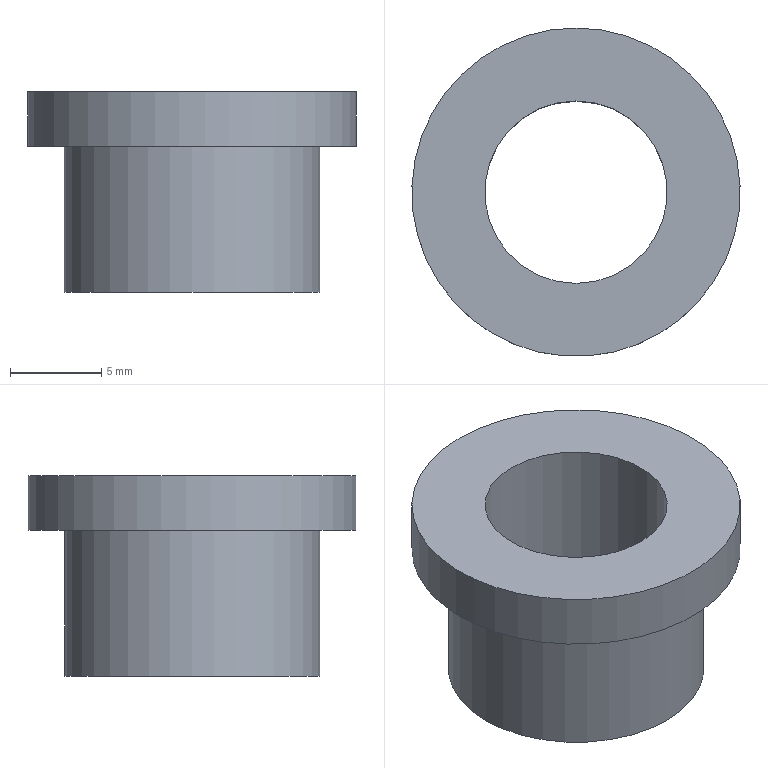Part | STEP file | 1-58A | 1 solid | 6 faces | box 18 x 18 x 11 mm | volume 1131 mm3 | plane 3 | cylinder 3 | commonest cylinder face diameters 10 x1 14 x1 18 x1
STEP:
#1=CARTESIAN_POINT('',(0.,0.,0.));
#2=DIRECTION('',(0.,0.,1.));
#3=DIRECTION('',(1.,0.,0.));
#4=AXIS2_PLACEMENT_3D('',#1,#2,#3);
#5=CARTESIAN_POINT('',(0.,7.,-8.));
#6=VERTEX_POINT('',#5);
#7=CARTESIAN_POINT('',(0.,0.,-8.));
#8=DIRECTION('',(0.,0.,1.));
#9=DIRECTION('',(0.,1.,0.));
#10=AXIS2_PLACEMENT_3D('',#7,#8,#9);
#11=CIRCLE('',#10,7.);
#12=CARTESIAN_POINT('',(0.,-1.876,-8.));
#13=DIRECTION('',(0.,0.,1.));
#14=DIRECTION('',(1.,0.,0.));
#15=AXIS2_PLACEMENT_3D('',#12,#13,#14);
#16=PLANE('',#15);
#17=CARTESIAN_POINT('',(0.,1.876));
#18=DIRECTION('',(0.,1.));
#19=AXIS2_PLACEMENT_2D('',#17,#18);
#20=CIRCLE('',#19,7.);
#21=(GEOMETRIC_REPRESENTATION_CONTEXT(2)PARAMETRIC_REPRESENTATION_CONTEXT()REPRESENTATION_CONTEXT('',''));
#22=DEFINITIONAL_REPRESENTATION('',(#20),#21);
#23=PCURVE('',#16,#22);
#24=CARTESIAN_POINT('',(0.,0.,0.));
#25=DIRECTION('',(0.,0.,-1.));
#26=DIRECTION('',(0.,1.,0.));
#27=AXIS2_PLACEMENT_3D('',#24,#25,#26);
#28=CYLINDRICAL_SURFACE('',#27,7.);
#29=CARTESIAN_POINT('',(6.283,8.));
#30=DIRECTION('',(-1.,0.));
#31=VECTOR('',#30,1.);
#32=LINE('',#29,#31);
#33=(GEOMETRIC_REPRESENTATION_CONTEXT(2)PARAMETRIC_REPRESENTATION_CONTEXT()REPRESENTATION_CONTEXT('',''));
#34=DEFINITIONAL_REPRESENTATION('',(#32),#33);
#35=PCURVE('',#28,#34);
#36=SURFACE_CURVE('',#11,(#23,#35),.PCURVE_S1.);
#37=EDGE_CURVE('',#6,#6,#36,.T.);
#38=ORIENTED_EDGE('',*,*,#37,.T.);
#39=EDGE_LOOP('',(#38));
#40=FACE_BOUND('',#39,.F.);
#41=CARTESIAN_POINT('',(0.,5.,-8.));
#42=VERTEX_POINT('',#41);
#43=CARTESIAN_POINT('',(0.,0.,-8.));
#44=DIRECTION('',(0.,0.,-1.));
#45=DIRECTION('',(0.,1.,0.));
#46=AXIS2_PLACEMENT_3D('',#43,#44,#45);
#47=CIRCLE('',#46,5.);
#48=CARTESIAN_POINT('',(0.,6.876));
#49=CARTESIAN_POINT('',(8.66,6.876));
#50=CARTESIAN_POINT('',(4.33,-0.6244));
#51=CARTESIAN_POINT('',(0.,-8.124));
#52=CARTESIAN_POINT('',(-4.33,-0.6244));
#53=CARTESIAN_POINT('',(-8.66,6.876));
#54=CARTESIAN_POINT('',(0.,6.876));
#55=(BOUNDED_CURVE()B_SPLINE_CURVE(2,(#48,#49,#50,#51,#52,#53,#54),.UNSPECIFIED.,.T.,.F.)B_SPLINE_CURVE_WITH_KNOTS((1,2,2,2,2,1),(-2.094,0.,2.094,4.189,6.283,8.378),.UNSPECIFIED.)CURVE()GEOMETRIC_REPRESENTATION_ITEM()RATIONAL_B_SPLINE_CURVE((1.,0.5,1.,0.5,1.,0.5,1.))REPRESENTATION_ITEM(''));
#56=(GEOMETRIC_REPRESENTATION_CONTEXT(2)PARAMETRIC_REPRESENTATION_CONTEXT()REPRESENTATION_CONTEXT('',''));
#57=DEFINITIONAL_REPRESENTATION('',(#55),#56);
#58=PCURVE('',#16,#57);
#59=CARTESIAN_POINT('',(0.,0.,3.));
#60=DIRECTION('',(0.,0.,-1.));
#61=DIRECTION('',(0.,1.,0.));
#62=AXIS2_PLACEMENT_3D('',#59,#60,#61);
#63=CYLINDRICAL_SURFACE('',#62,5.);
#64=CARTESIAN_POINT('',(0.,11.));
#65=DIRECTION('',(1.,0.));
#66=VECTOR('',#65,1.);
#67=LINE('',#64,#66);
#68=(GEOMETRIC_REPRESENTATION_CONTEXT(2)PARAMETRIC_REPRESENTATION_CONTEXT()REPRESENTATION_CONTEXT('',''));
#69=DEFINITIONAL_REPRESENTATION('',(#67),#68);
#70=PCURVE('',#63,#69);
#71=SURFACE_CURVE('',#47,(#58,#70),.PCURVE_S1.);
#72=EDGE_CURVE('',#42,#42,#71,.T.);
#73=ORIENTED_EDGE('',*,*,#72,.T.);
#74=EDGE_LOOP('',(#73));
#75=FACE_BOUND('',#74,.F.);
#76=ADVANCED_FACE('',(#40,#75),#16,.F.);
#77=CARTESIAN_POINT('',(0.,7.,0.));
#78=VERTEX_POINT('',#77);
#79=CARTESIAN_POINT('',(0.,7.,0.));
#80=DIRECTION('',(0.,0.,-1.));
#81=VECTOR('',#80,1.);
#82=LINE('',#79,#81);
#83=CARTESIAN_POINT('',(6.283,0.));
#84=DIRECTION('',(0.,1.));
#85=VECTOR('',#84,1.);
#86=LINE('',#83,#85);
#87=(GEOMETRIC_REPRESENTATION_CONTEXT(2)PARAMETRIC_REPRESENTATION_CONTEXT()REPRESENTATION_CONTEXT('',''));
#88=DEFINITIONAL_REPRESENTATION('',(#86),#87);
#89=PCURVE('',#28,#88);
#90=CARTESIAN_POINT('',(0.,0.));
#91=DIRECTION('',(0.,1.));
#92=VECTOR('',#91,1.);
#93=LINE('',#90,#92);
#94=(GEOMETRIC_REPRESENTATION_CONTEXT(2)PARAMETRIC_REPRESENTATION_CONTEXT()REPRESENTATION_CONTEXT('',''));
#95=DEFINITIONAL_REPRESENTATION('',(#93),#94);
#96=PCURVE('',#28,#95);
#97=SEAM_CURVE('',#82,(#89,#96),.PCURVE_S1.);
#98=EDGE_CURVE('',#78,#6,#97,.T.);
#99=ORIENTED_EDGE('',*,*,#98,.T.);
#100=ORIENTED_EDGE('',*,*,#37,.T.);
#101=ORIENTED_EDGE('',*,*,#98,.F.);
#102=CARTESIAN_POINT('',(0.,0.,0.));
#103=DIRECTION('',(0.,0.,1.));
#104=DIRECTION('',(0.,1.,0.));
#105=AXIS2_PLACEMENT_3D('',#102,#103,#104);
#106=CIRCLE('',#105,7.);
#107=CARTESIAN_POINT('',(6.283,0.));
#108=DIRECTION('',(-1.,0.));
#109=VECTOR('',#108,1.);
#110=LINE('',#107,#109);
#111=(GEOMETRIC_REPRESENTATION_CONTEXT(2)PARAMETRIC_REPRESENTATION_CONTEXT()REPRESENTATION_CONTEXT('',''));
#112=DEFINITIONAL_REPRESENTATION('',(#110),#111);
#113=PCURVE('',#28,#112);
#114=CARTESIAN_POINT('',(0.,-2.412,0.));
#115=DIRECTION('',(0.,0.,1.));
#116=DIRECTION('',(1.,0.,0.));
#117=AXIS2_PLACEMENT_3D('',#114,#115,#116);
#118=PLANE('',#117);
#119=CARTESIAN_POINT('',(0.,2.412));
#120=DIRECTION('',(0.,1.));
#121=AXIS2_PLACEMENT_2D('',#119,#120);
#122=CIRCLE('',#121,7.);
#123=(GEOMETRIC_REPRESENTATION_CONTEXT(2)PARAMETRIC_REPRESENTATION_CONTEXT()REPRESENTATION_CONTEXT('',''));
#124=DEFINITIONAL_REPRESENTATION('',(#122),#123);
#125=PCURVE('',#118,#124);
#126=SURFACE_CURVE('',#106,(#113,#125),.PCURVE_S1.);
#127=EDGE_CURVE('',#78,#78,#126,.T.);
#128=ORIENTED_EDGE('',*,*,#127,.F.);
#129=EDGE_LOOP('',(#99,#100,#101,#128));
#130=FACE_BOUND('',#129,.T.);
#131=ADVANCED_FACE('',(#130),#28,.T.);
#132=ORIENTED_EDGE('',*,*,#72,.F.);
#133=CARTESIAN_POINT('',(0.,5.,3.));
#134=VERTEX_POINT('',#133);
#135=CARTESIAN_POINT('',(0.,5.,-8.));
#136=DIRECTION('',(0.,0.,1.));
#137=VECTOR('',#136,1.);
#138=LINE('',#135,#137);
#139=CARTESIAN_POINT('',(0.,11.));
#140=DIRECTION('',(0.,-1.));
#141=VECTOR('',#140,1.);
#142=LINE('',#139,#141);
#143=(GEOMETRIC_REPRESENTATION_CONTEXT(2)PARAMETRIC_REPRESENTATION_CONTEXT()REPRESENTATION_CONTEXT('',''));
#144=DEFINITIONAL_REPRESENTATION('',(#142),#143);
#145=PCURVE('',#63,#144);
#146=CARTESIAN_POINT('',(6.283,11.));
#147=DIRECTION('',(0.,-1.));
#148=VECTOR('',#147,1.);
#149=LINE('',#146,#148);
#150=(GEOMETRIC_REPRESENTATION_CONTEXT(2)PARAMETRIC_REPRESENTATION_CONTEXT()REPRESENTATION_CONTEXT('',''));
#151=DEFINITIONAL_REPRESENTATION('',(#149),#150);
#152=PCURVE('',#63,#151);
#153=SEAM_CURVE('',#138,(#145,#152),.PCURVE_S1.);
#154=EDGE_CURVE('',#42,#134,#153,.T.);
#155=ORIENTED_EDGE('',*,*,#154,.T.);
#156=CARTESIAN_POINT('',(0.,0.,3.));
#157=DIRECTION('',(0.,0.,-1.));
#158=DIRECTION('',(0.,1.,0.));
#159=AXIS2_PLACEMENT_3D('',#156,#157,#158);
#160=CIRCLE('',#159,5.);
#161=CARTESIAN_POINT('',(0.,0.));
#162=DIRECTION('',(1.,0.));
#163=VECTOR('',#162,1.);
#164=LINE('',#161,#163);
#165=(GEOMETRIC_REPRESENTATION_CONTEXT(2)PARAMETRIC_REPRESENTATION_CONTEXT()REPRESENTATION_CONTEXT('',''));
#166=DEFINITIONAL_REPRESENTATION('',(#164),#165);
#167=PCURVE('',#63,#166);
#168=CARTESIAN_POINT('',(0.,-2.412,3.));
#169=DIRECTION('',(0.,0.,1.));
#170=DIRECTION('',(1.,0.,0.));
#171=AXIS2_PLACEMENT_3D('',#168,#169,#170);
#172=PLANE('',#171);
#173=CARTESIAN_POINT('',(0.,7.412));
#174=CARTESIAN_POINT('',(8.66,7.412));
#175=CARTESIAN_POINT('',(4.33,-0.08846));
#176=CARTESIAN_POINT('',(0.,-7.588));
#177=CARTESIAN_POINT('',(-4.33,-0.08846));
#178=CARTESIAN_POINT('',(-8.66,7.412));
#179=CARTESIAN_POINT('',(0.,7.412));
#180=(BOUNDED_CURVE()B_SPLINE_CURVE(2,(#173,#174,#175,#176,#177,#178,#179),.UNSPECIFIED.,.T.,.F.)B_SPLINE_CURVE_WITH_KNOTS((1,2,2,2,2,1),(-2.094,0.,2.094,4.189,6.283,8.378),.UNSPECIFIED.)CURVE()GEOMETRIC_REPRESENTATION_ITEM()RATIONAL_B_SPLINE_CURVE((1.,0.5,1.,0.5,1.,0.5,1.))REPRESENTATION_ITEM(''));
#181=(GEOMETRIC_REPRESENTATION_CONTEXT(2)PARAMETRIC_REPRESENTATION_CONTEXT()REPRESENTATION_CONTEXT('',''));
#182=DEFINITIONAL_REPRESENTATION('',(#180),#181);
#183=PCURVE('',#172,#182);
#184=SURFACE_CURVE('',#160,(#167,#183),.PCURVE_S1.);
#185=EDGE_CURVE('',#134,#134,#184,.T.);
#186=ORIENTED_EDGE('',*,*,#185,.T.);
#187=ORIENTED_EDGE('',*,*,#154,.F.);
#188=EDGE_LOOP('',(#132,#155,#186,#187));
#189=FACE_BOUND('',#188,.F.);
#190=ADVANCED_FACE('',(#189),#63,.F.);
#191=CARTESIAN_POINT('',(0.,9.,0.));
#192=VERTEX_POINT('',#191);
#193=CARTESIAN_POINT('',(0.,0.,0.));
#194=DIRECTION('',(0.,0.,1.));
#195=DIRECTION('',(0.,1.,0.));
#196=AXIS2_PLACEMENT_3D('',#193,#194,#195);
#197=CIRCLE('',#196,9.);
#198=CARTESIAN_POINT('',(0.,2.412));
#199=DIRECTION('',(0.,1.));
#200=AXIS2_PLACEMENT_2D('',#198,#199);
#201=CIRCLE('',#200,9.);
#202=(GEOMETRIC_REPRESENTATION_CONTEXT(2)PARAMETRIC_REPRESENTATION_CONTEXT()REPRESENTATION_CONTEXT('',''));
#203=DEFINITIONAL_REPRESENTATION('',(#201),#202);
#204=PCURVE('',#118,#203);
#205=CARTESIAN_POINT('',(0.,0.,0.));
#206=DIRECTION('',(0.,0.,1.));
#207=DIRECTION('',(0.,1.,0.));
#208=AXIS2_PLACEMENT_3D('',#205,#206,#207);
#209=CYLINDRICAL_SURFACE('',#208,9.);
#210=CARTESIAN_POINT('',(0.,0.));
#211=DIRECTION('',(1.,0.));
#212=VECTOR('',#211,1.);
#213=LINE('',#210,#212);
#214=(GEOMETRIC_REPRESENTATION_CONTEXT(2)PARAMETRIC_REPRESENTATION_CONTEXT()REPRESENTATION_CONTEXT('',''));
#215=DEFINITIONAL_REPRESENTATION('',(#213),#214);
#216=PCURVE('',#209,#215);
#217=SURFACE_CURVE('',#197,(#204,#216),.PCURVE_S1.);
#218=EDGE_CURVE('',#192,#192,#217,.T.);
#219=ORIENTED_EDGE('',*,*,#218,.T.);
#220=EDGE_LOOP('',(#219));
#221=FACE_BOUND('',#220,.F.);
#222=ORIENTED_EDGE('',*,*,#127,.F.);
#223=EDGE_LOOP('',(#222));
#224=FACE_BOUND('',#223,.F.);
#225=ADVANCED_FACE('',(#221,#224),#118,.F.);
#226=ORIENTED_EDGE('',*,*,#218,.T.);
#227=CARTESIAN_POINT('',(0.,9.,3.));
#228=VERTEX_POINT('',#227);
#229=CARTESIAN_POINT('',(0.,9.,0.));
#230=DIRECTION('',(0.,0.,1.));
#231=VECTOR('',#230,1.);
#232=LINE('',#229,#231);
#233=CARTESIAN_POINT('',(6.283,0.));
#234=DIRECTION('',(0.,1.));
#235=VECTOR('',#234,1.);
#236=LINE('',#233,#235);
#237=(GEOMETRIC_REPRESENTATION_CONTEXT(2)PARAMETRIC_REPRESENTATION_CONTEXT()REPRESENTATION_CONTEXT('',''));
#238=DEFINITIONAL_REPRESENTATION('',(#236),#237);
#239=PCURVE('',#209,#238);
#240=CARTESIAN_POINT('',(0.,0.));
#241=DIRECTION('',(0.,1.));
#242=VECTOR('',#241,1.);
#243=LINE('',#240,#242);
#244=(GEOMETRIC_REPRESENTATION_CONTEXT(2)PARAMETRIC_REPRESENTATION_CONTEXT()REPRESENTATION_CONTEXT('',''));
#245=DEFINITIONAL_REPRESENTATION('',(#243),#244);
#246=PCURVE('',#209,#245);
#247=SEAM_CURVE('',#232,(#239,#246),.PCURVE_S1.);
#248=EDGE_CURVE('',#192,#228,#247,.T.);
#249=ORIENTED_EDGE('',*,*,#248,.T.);
#250=CARTESIAN_POINT('',(0.,0.,3.));
#251=DIRECTION('',(0.,0.,1.));
#252=DIRECTION('',(0.,1.,0.));
#253=AXIS2_PLACEMENT_3D('',#250,#251,#252);
#254=CIRCLE('',#253,9.);
#255=CARTESIAN_POINT('',(0.,3.));
#256=DIRECTION('',(1.,0.));
#257=VECTOR('',#256,1.);
#258=LINE('',#255,#257);
#259=(GEOMETRIC_REPRESENTATION_CONTEXT(2)PARAMETRIC_REPRESENTATION_CONTEXT()REPRESENTATION_CONTEXT('',''));
#260=DEFINITIONAL_REPRESENTATION('',(#258),#259);
#261=PCURVE('',#209,#260);
#262=CARTESIAN_POINT('',(0.,2.412));
#263=DIRECTION('',(0.,1.));
#264=AXIS2_PLACEMENT_2D('',#262,#263);
#265=CIRCLE('',#264,9.);
#266=(GEOMETRIC_REPRESENTATION_CONTEXT(2)PARAMETRIC_REPRESENTATION_CONTEXT()REPRESENTATION_CONTEXT('',''));
#267=DEFINITIONAL_REPRESENTATION('',(#265),#266);
#268=PCURVE('',#172,#267);
#269=SURFACE_CURVE('',#254,(#261,#268),.PCURVE_S1.);
#270=EDGE_CURVE('',#228,#228,#269,.T.);
#271=ORIENTED_EDGE('',*,*,#270,.F.);
#272=ORIENTED_EDGE('',*,*,#248,.F.);
#273=EDGE_LOOP('',(#226,#249,#271,#272));
#274=FACE_BOUND('',#273,.T.);
#275=ADVANCED_FACE('',(#274),#209,.T.);
#276=ORIENTED_EDGE('',*,*,#270,.T.);
#277=EDGE_LOOP('',(#276));
#278=FACE_BOUND('',#277,.T.);
#279=ORIENTED_EDGE('',*,*,#185,.T.);
#280=EDGE_LOOP('',(#279));
#281=FACE_BOUND('',#280,.T.);
#282=ADVANCED_FACE('',(#278,#281),#172,.T.);
#283=CLOSED_SHELL('',(#76,#131,#190,#225,#275,#282));
#284=MANIFOLD_SOLID_BREP('',#283);
#285=(LENGTH_UNIT()NAMED_UNIT(*)SI_UNIT(.MILLI.,.METRE.));
#286=UNCERTAINTY_MEASURE_WITH_UNIT(LENGTH_MEASURE(0.0000001),#285,'','');
#287=(NAMED_UNIT(*)PLANE_ANGLE_UNIT()SI_UNIT($,.RADIAN.));
#288=(NAMED_UNIT(*)SI_UNIT($,.STERADIAN.)SOLID_ANGLE_UNIT());
#289=(GEOMETRIC_REPRESENTATION_CONTEXT(3)GLOBAL_UNCERTAINTY_ASSIGNED_CONTEXT((#286))GLOBAL_UNIT_ASSIGNED_CONTEXT((#285,#287,#288))REPRESENTATION_CONTEXT('',''));
#290=ADVANCED_BREP_SHAPE_REPRESENTATION('',(#4,#284),#289);